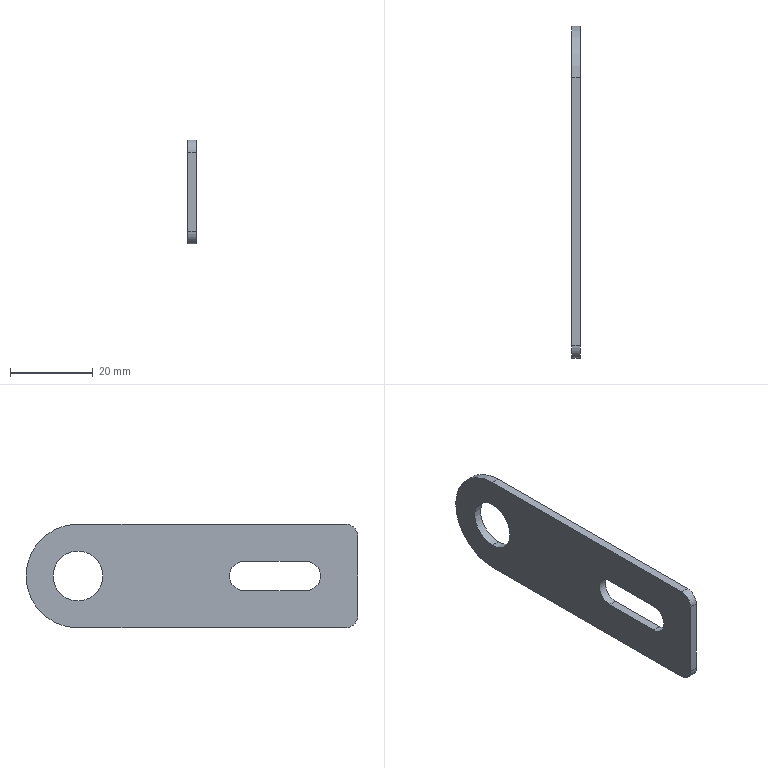Part | STEP file | Proximity switch bracket 1 | 1 solid | 15 faces | box 2 x 80 x 25 mm | volume 3345 mm3 | cylinder 8 | plane 7 | commonest cylinder face diameters 6 x2 7 x2 12 x2 25 x2
STEP:
#1=CARTESIAN_POINT('',(0.,0.,0.));
#2=DIRECTION('',(0.,0.,1.));
#3=DIRECTION('',(1.,0.,0.));
#4=AXIS2_PLACEMENT_3D('',#1,#2,#3);
#5=CARTESIAN_POINT('',(0.,67.5,6.));
#6=VERTEX_POINT('',#5);
#7=CARTESIAN_POINT('',(-2.,67.5,6.));
#8=VERTEX_POINT('',#7);
#9=CARTESIAN_POINT('',(-2.,67.5,6.));
#10=DIRECTION('',(-1.,0.,0.));
#11=VECTOR('',#10,1.);
#12=LINE('',#9,#11);
#13=CARTESIAN_POINT('',(-2.,67.5,0.));
#14=DIRECTION('',(-1.,0.,0.));
#15=DIRECTION('',(0.,0.,1.));
#16=AXIS2_PLACEMENT_3D('',#13,#14,#15);
#17=CYLINDRICAL_SURFACE('',#16,6.);
#18=CARTESIAN_POINT('',(6.283,0.));
#19=DIRECTION('',(0.,1.));
#20=VECTOR('',#19,1.);
#21=LINE('',#18,#20);
#22=(GEOMETRIC_REPRESENTATION_CONTEXT(2)PARAMETRIC_REPRESENTATION_CONTEXT()REPRESENTATION_CONTEXT('',''));
#23=DEFINITIONAL_REPRESENTATION('',(#21),#22);
#24=PCURVE('',#17,#23);
#25=CARTESIAN_POINT('',(-2.,67.5,0.));
#26=DIRECTION('',(-1.,0.,0.));
#27=DIRECTION('',(0.,0.,1.));
#28=AXIS2_PLACEMENT_3D('',#25,#26,#27);
#29=CYLINDRICAL_SURFACE('',#28,6.);
#30=CARTESIAN_POINT('',(0.,0.));
#31=DIRECTION('',(0.,1.));
#32=VECTOR('',#31,1.);
#33=LINE('',#30,#32);
#34=(GEOMETRIC_REPRESENTATION_CONTEXT(2)PARAMETRIC_REPRESENTATION_CONTEXT()REPRESENTATION_CONTEXT('',''));
#35=DEFINITIONAL_REPRESENTATION('',(#33),#34);
#36=PCURVE('',#29,#35);
#37=SURFACE_CURVE('',#12,(#24,#36),.PCURVE_S1.);
#38=EDGE_CURVE('',#6,#8,#37,.T.);
#39=ORIENTED_EDGE('',*,*,#38,.T.);
#40=CARTESIAN_POINT('',(-2.,67.5,-6.));
#41=VERTEX_POINT('',#40);
#42=CARTESIAN_POINT('',(-2.,67.5,0.));
#43=DIRECTION('',(-1.,0.,0.));
#44=DIRECTION('',(0.,0.,1.));
#45=AXIS2_PLACEMENT_3D('',#42,#43,#44);
#46=CIRCLE('',#45,6.);
#47=CARTESIAN_POINT('',(0.,0.));
#48=DIRECTION('',(1.,0.));
#49=VECTOR('',#48,1.);
#50=LINE('',#47,#49);
#51=(GEOMETRIC_REPRESENTATION_CONTEXT(2)PARAMETRIC_REPRESENTATION_CONTEXT()REPRESENTATION_CONTEXT('',''));
#52=DEFINITIONAL_REPRESENTATION('',(#50),#51);
#53=PCURVE('',#17,#52);
#54=CARTESIAN_POINT('',(-2.,0.,12.5));
#55=DIRECTION('',(1.,0.,0.));
#56=DIRECTION('',(0.,0.,-1.));
#57=AXIS2_PLACEMENT_3D('',#54,#55,#56);
#58=PLANE('',#57);
#59=CARTESIAN_POINT('',(6.5,67.5));
#60=CARTESIAN_POINT('',(6.5,77.892));
#61=CARTESIAN_POINT('',(15.5,72.696));
#62=CARTESIAN_POINT('',(24.5,67.5));
#63=CARTESIAN_POINT('',(15.5,62.304));
#64=CARTESIAN_POINT('',(6.5,57.108));
#65=CARTESIAN_POINT('',(6.5,67.5));
#66=(BOUNDED_CURVE()B_SPLINE_CURVE(2,(#59,#60,#61,#62,#63,#64,#65),.UNSPECIFIED.,.T.,.F.)B_SPLINE_CURVE_WITH_KNOTS((1,2,2,2,2,1),(-2.094,0.,2.094,4.189,6.283,8.378),.UNSPECIFIED.)CURVE()GEOMETRIC_REPRESENTATION_ITEM()RATIONAL_B_SPLINE_CURVE((1.,0.5,1.,0.5,1.,0.5,1.))REPRESENTATION_ITEM(''));
#67=(GEOMETRIC_REPRESENTATION_CONTEXT(2)PARAMETRIC_REPRESENTATION_CONTEXT()REPRESENTATION_CONTEXT('',''));
#68=DEFINITIONAL_REPRESENTATION('',(#66),#67);
#69=PCURVE('',#58,#68);
#70=SURFACE_CURVE('',#46,(#53,#69),.PCURVE_S1.);
#71=EDGE_CURVE('',#41,#8,#70,.T.);
#72=ORIENTED_EDGE('',*,*,#71,.F.);
#73=CARTESIAN_POINT('',(0.,67.5,-6.));
#74=VERTEX_POINT('',#73);
#75=CARTESIAN_POINT('',(-2.,67.5,-6.));
#76=DIRECTION('',(-1.,0.,0.));
#77=VECTOR('',#76,1.);
#78=LINE('',#75,#77);
#79=CARTESIAN_POINT('',(3.142,0.));
#80=DIRECTION('',(0.,1.));
#81=VECTOR('',#80,1.);
#82=LINE('',#79,#81);
#83=(GEOMETRIC_REPRESENTATION_CONTEXT(2)PARAMETRIC_REPRESENTATION_CONTEXT()REPRESENTATION_CONTEXT('',''));
#84=DEFINITIONAL_REPRESENTATION('',(#82),#83);
#85=PCURVE('',#17,#84);
#86=CARTESIAN_POINT('',(3.142,0.));
#87=DIRECTION('',(0.,1.));
#88=VECTOR('',#87,1.);
#89=LINE('',#86,#88);
#90=(GEOMETRIC_REPRESENTATION_CONTEXT(2)PARAMETRIC_REPRESENTATION_CONTEXT()REPRESENTATION_CONTEXT('',''));
#91=DEFINITIONAL_REPRESENTATION('',(#89),#90);
#92=PCURVE('',#29,#91);
#93=SURFACE_CURVE('',#78,(#85,#92),.PCURVE_S1.);
#94=EDGE_CURVE('',#74,#41,#93,.T.);
#95=ORIENTED_EDGE('',*,*,#94,.F.);
#96=CARTESIAN_POINT('',(0.,67.5,0.));
#97=DIRECTION('',(-1.,0.,0.));
#98=DIRECTION('',(0.,0.,1.));
#99=AXIS2_PLACEMENT_3D('',#96,#97,#98);
#100=CIRCLE('',#99,6.);
#101=CARTESIAN_POINT('',(0.,-2.));
#102=DIRECTION('',(1.,0.));
#103=VECTOR('',#102,1.);
#104=LINE('',#101,#103);
#105=(GEOMETRIC_REPRESENTATION_CONTEXT(2)PARAMETRIC_REPRESENTATION_CONTEXT()REPRESENTATION_CONTEXT('',''));
#106=DEFINITIONAL_REPRESENTATION('',(#104),#105);
#107=PCURVE('',#17,#106);
#108=CARTESIAN_POINT('',(0.,0.,12.5));
#109=DIRECTION('',(1.,0.,0.));
#110=DIRECTION('',(0.,0.,-1.));
#111=AXIS2_PLACEMENT_3D('',#108,#109,#110);
#112=PLANE('',#111);
#113=CARTESIAN_POINT('',(6.5,67.5));
#114=CARTESIAN_POINT('',(6.5,77.892));
#115=CARTESIAN_POINT('',(15.5,72.696));
#116=CARTESIAN_POINT('',(24.5,67.5));
#117=CARTESIAN_POINT('',(15.5,62.304));
#118=CARTESIAN_POINT('',(6.5,57.108));
#119=CARTESIAN_POINT('',(6.5,67.5));
#120=(BOUNDED_CURVE()B_SPLINE_CURVE(2,(#113,#114,#115,#116,#117,#118,#119),.UNSPECIFIED.,.T.,.F.)B_SPLINE_CURVE_WITH_KNOTS((1,2,2,2,2,1),(-2.094,0.,2.094,4.189,6.283,8.378),.UNSPECIFIED.)CURVE()GEOMETRIC_REPRESENTATION_ITEM()RATIONAL_B_SPLINE_CURVE((1.,0.5,1.,0.5,1.,0.5,1.))REPRESENTATION_ITEM(''));
#121=(GEOMETRIC_REPRESENTATION_CONTEXT(2)PARAMETRIC_REPRESENTATION_CONTEXT()REPRESENTATION_CONTEXT('',''));
#122=DEFINITIONAL_REPRESENTATION('',(#120),#121);
#123=PCURVE('',#112,#122);
#124=SURFACE_CURVE('',#100,(#107,#123),.PCURVE_S1.);
#125=EDGE_CURVE('',#74,#6,#124,.T.);
#126=ORIENTED_EDGE('',*,*,#125,.T.);
#127=EDGE_LOOP('',(#39,#72,#95,#126));
#128=FACE_BOUND('',#127,.F.);
#129=ADVANCED_FACE('',(#128),#17,.F.);
#130=CARTESIAN_POINT('',(-2.,12.5,3.5));
#131=VERTEX_POINT('',#130);
#132=CARTESIAN_POINT('',(-2.,27.5,3.5));
#133=VERTEX_POINT('',#132);
#134=CARTESIAN_POINT('',(-2.,12.5,3.5));
#135=DIRECTION('',(0.,1.,0.));
#136=VECTOR('',#135,1.);
#137=LINE('',#134,#136);
#138=CARTESIAN_POINT('',(9.,12.5));
#139=DIRECTION('',(0.,1.));
#140=VECTOR('',#139,1.);
#141=LINE('',#138,#140);
#142=(GEOMETRIC_REPRESENTATION_CONTEXT(2)PARAMETRIC_REPRESENTATION_CONTEXT()REPRESENTATION_CONTEXT('',''));
#143=DEFINITIONAL_REPRESENTATION('',(#141),#142);
#144=PCURVE('',#58,#143);
#145=CARTESIAN_POINT('',(0.,12.5,3.5));
#146=DIRECTION('',(0.,0.,1.));
#147=DIRECTION('',(0.,-1.,0.));
#148=AXIS2_PLACEMENT_3D('',#145,#146,#147);
#149=PLANE('',#148);
#150=CARTESIAN_POINT('',(0.,-2.));
#151=DIRECTION('',(-1.,0.));
#152=VECTOR('',#151,1.);
#153=LINE('',#150,#152);
#154=(GEOMETRIC_REPRESENTATION_CONTEXT(2)PARAMETRIC_REPRESENTATION_CONTEXT()REPRESENTATION_CONTEXT('',''));
#155=DEFINITIONAL_REPRESENTATION('',(#153),#154);
#156=PCURVE('',#149,#155);
#157=SURFACE_CURVE('',#137,(#144,#156),.PCURVE_S1.);
#158=EDGE_CURVE('',#131,#133,#157,.T.);
#159=ORIENTED_EDGE('',*,*,#158,.F.);
#160=CARTESIAN_POINT('',(-2.,12.5,-3.5));
#161=VERTEX_POINT('',#160);
#162=CARTESIAN_POINT('',(-2.,12.5,0.));
#163=DIRECTION('',(-1.,0.,0.));
#164=DIRECTION('',(0.,0.,1.));
#165=AXIS2_PLACEMENT_3D('',#162,#163,#164);
#166=CIRCLE('',#165,3.5);
#167=CARTESIAN_POINT('',(9.,12.5));
#168=CARTESIAN_POINT('',(9.,18.562));
#169=CARTESIAN_POINT('',(14.25,15.531));
#170=CARTESIAN_POINT('',(19.5,12.5));
#171=CARTESIAN_POINT('',(14.25,9.469));
#172=CARTESIAN_POINT('',(9.,6.438));
#173=CARTESIAN_POINT('',(9.,12.5));
#174=(BOUNDED_CURVE()B_SPLINE_CURVE(2,(#167,#168,#169,#170,#171,#172,#173),.UNSPECIFIED.,.T.,.F.)B_SPLINE_CURVE_WITH_KNOTS((1,2,2,2,2,1),(-2.094,0.,2.094,4.189,6.283,8.378),.UNSPECIFIED.)CURVE()GEOMETRIC_REPRESENTATION_ITEM()RATIONAL_B_SPLINE_CURVE((1.,0.5,1.,0.5,1.,0.5,1.))REPRESENTATION_ITEM(''));
#175=(GEOMETRIC_REPRESENTATION_CONTEXT(2)PARAMETRIC_REPRESENTATION_CONTEXT()REPRESENTATION_CONTEXT('',''));
#176=DEFINITIONAL_REPRESENTATION('',(#174),#175);
#177=PCURVE('',#58,#176);
#178=CARTESIAN_POINT('',(0.,12.5,0.));
#179=DIRECTION('',(-1.,0.,0.));
#180=DIRECTION('',(0.,0.,1.));
#181=AXIS2_PLACEMENT_3D('',#178,#179,#180);
#182=CYLINDRICAL_SURFACE('',#181,3.5);
#183=CARTESIAN_POINT('',(0.,2.));
#184=DIRECTION('',(1.,0.));
#185=VECTOR('',#184,1.);
#186=LINE('',#183,#185);
#187=(GEOMETRIC_REPRESENTATION_CONTEXT(2)PARAMETRIC_REPRESENTATION_CONTEXT()REPRESENTATION_CONTEXT('',''));
#188=DEFINITIONAL_REPRESENTATION('',(#186),#187);
#189=PCURVE('',#182,#188);
#190=SURFACE_CURVE('',#166,(#177,#189),.PCURVE_S1.);
#191=EDGE_CURVE('',#161,#131,#190,.T.);
#192=ORIENTED_EDGE('',*,*,#191,.F.);
#193=CARTESIAN_POINT('',(-2.,27.5,-3.5));
#194=VERTEX_POINT('',#193);
#195=CARTESIAN_POINT('',(-2.,12.5,-3.5));
#196=DIRECTION('',(0.,-1.,0.));
#197=VECTOR('',#196,1.);
#198=LINE('',#195,#197);
#199=CARTESIAN_POINT('',(16.,12.5));
#200=DIRECTION('',(0.,-1.));
#201=VECTOR('',#200,1.);
#202=LINE('',#199,#201);
#203=(GEOMETRIC_REPRESENTATION_CONTEXT(2)PARAMETRIC_REPRESENTATION_CONTEXT()REPRESENTATION_CONTEXT('',''));
#204=DEFINITIONAL_REPRESENTATION('',(#202),#203);
#205=PCURVE('',#58,#204);
#206=CARTESIAN_POINT('',(0.,12.5,-3.5));
#207=DIRECTION('',(0.,0.,-1.));
#208=DIRECTION('',(0.,1.,0.));
#209=AXIS2_PLACEMENT_3D('',#206,#207,#208);
#210=PLANE('',#209);
#211=CARTESIAN_POINT('',(0.,-2.));
#212=DIRECTION('',(-1.,0.));
#213=VECTOR('',#212,1.);
#214=LINE('',#211,#213);
#215=(GEOMETRIC_REPRESENTATION_CONTEXT(2)PARAMETRIC_REPRESENTATION_CONTEXT()REPRESENTATION_CONTEXT('',''));
#216=DEFINITIONAL_REPRESENTATION('',(#214),#215);
#217=PCURVE('',#210,#216);
#218=SURFACE_CURVE('',#198,(#205,#217),.PCURVE_S1.);
#219=EDGE_CURVE('',#194,#161,#218,.T.);
#220=ORIENTED_EDGE('',*,*,#219,.F.);
#221=CARTESIAN_POINT('',(-2.,27.5,0.));
#222=DIRECTION('',(-1.,0.,0.));
#223=DIRECTION('',(0.,0.,1.));
#224=AXIS2_PLACEMENT_3D('',#221,#222,#223);
#225=CIRCLE('',#224,3.5);
#226=CARTESIAN_POINT('',(9.,27.5));
#227=CARTESIAN_POINT('',(9.,33.562));
#228=CARTESIAN_POINT('',(14.25,30.531));
#229=CARTESIAN_POINT('',(19.5,27.5));
#230=CARTESIAN_POINT('',(14.25,24.469));
#231=CARTESIAN_POINT('',(9.,21.438));
#232=CARTESIAN_POINT('',(9.,27.5));
#233=(BOUNDED_CURVE()B_SPLINE_CURVE(2,(#226,#227,#228,#229,#230,#231,#232),.UNSPECIFIED.,.T.,.F.)B_SPLINE_CURVE_WITH_KNOTS((1,2,2,2,2,1),(-2.094,0.,2.094,4.189,6.283,8.378),.UNSPECIFIED.)CURVE()GEOMETRIC_REPRESENTATION_ITEM()RATIONAL_B_SPLINE_CURVE((1.,0.5,1.,0.5,1.,0.5,1.))REPRESENTATION_ITEM(''));
#234=(GEOMETRIC_REPRESENTATION_CONTEXT(2)PARAMETRIC_REPRESENTATION_CONTEXT()REPRESENTATION_CONTEXT('',''));
#235=DEFINITIONAL_REPRESENTATION('',(#233),#234);
#236=PCURVE('',#58,#235);
#237=CARTESIAN_POINT('',(0.,27.5,0.));
#238=DIRECTION('',(-1.,0.,0.));
#239=DIRECTION('',(0.,0.,1.));
#240=AXIS2_PLACEMENT_3D('',#237,#238,#239);
#241=CYLINDRICAL_SURFACE('',#240,3.5);
#242=CARTESIAN_POINT('',(0.,2.));
#243=DIRECTION('',(1.,0.));
#244=VECTOR('',#243,1.);
#245=LINE('',#242,#244);
#246=(GEOMETRIC_REPRESENTATION_CONTEXT(2)PARAMETRIC_REPRESENTATION_CONTEXT()REPRESENTATION_CONTEXT('',''));
#247=DEFINITIONAL_REPRESENTATION('',(#245),#246);
#248=PCURVE('',#241,#247);
#249=SURFACE_CURVE('',#225,(#236,#248),.PCURVE_S1.);
#250=EDGE_CURVE('',#133,#194,#249,.T.);
#251=ORIENTED_EDGE('',*,*,#250,.F.);
#252=EDGE_LOOP('',(#159,#192,#220,#251));
#253=FACE_BOUND('',#252,.T.);
#254=CARTESIAN_POINT('',(-2.,67.5,0.));
#255=DIRECTION('',(-1.,0.,0.));
#256=DIRECTION('',(0.,0.,1.));
#257=AXIS2_PLACEMENT_3D('',#254,#255,#256);
#258=CIRCLE('',#257,6.);
#259=CARTESIAN_POINT('',(6.5,67.5));
#260=CARTESIAN_POINT('',(6.5,77.892));
#261=CARTESIAN_POINT('',(15.5,72.696));
#262=CARTESIAN_POINT('',(24.5,67.5));
#263=CARTESIAN_POINT('',(15.5,62.304));
#264=CARTESIAN_POINT('',(6.5,57.108));
#265=CARTESIAN_POINT('',(6.5,67.5));
#266=(BOUNDED_CURVE()B_SPLINE_CURVE(2,(#259,#260,#261,#262,#263,#264,#265),.UNSPECIFIED.,.T.,.F.)B_SPLINE_CURVE_WITH_KNOTS((1,2,2,2,2,1),(-2.094,0.,2.094,4.189,6.283,8.378),.UNSPECIFIED.)CURVE()GEOMETRIC_REPRESENTATION_ITEM()RATIONAL_B_SPLINE_CURVE((1.,0.5,1.,0.5,1.,0.5,1.))REPRESENTATION_ITEM(''));
#267=(GEOMETRIC_REPRESENTATION_CONTEXT(2)PARAMETRIC_REPRESENTATION_CONTEXT()REPRESENTATION_CONTEXT('',''));
#268=DEFINITIONAL_REPRESENTATION('',(#266),#267);
#269=PCURVE('',#58,#268);
#270=CARTESIAN_POINT('',(0.,0.));
#271=DIRECTION('',(1.,0.));
#272=VECTOR('',#271,1.);
#273=LINE('',#270,#272);
#274=(GEOMETRIC_REPRESENTATION_CONTEXT(2)PARAMETRIC_REPRESENTATION_CONTEXT()REPRESENTATION_CONTEXT('',''));
#275=DEFINITIONAL_REPRESENTATION('',(#273),#274);
#276=PCURVE('',#29,#275);
#277=SURFACE_CURVE('',#258,(#269,#276),.PCURVE_S1.);
#278=EDGE_CURVE('',#8,#41,#277,.T.);
#279=ORIENTED_EDGE('',*,*,#278,.F.);
#280=ORIENTED_EDGE('',*,*,#71,.F.);
#281=EDGE_LOOP('',(#279,#280));
#282=FACE_BOUND('',#281,.T.);
#283=CARTESIAN_POINT('',(-2.,0.,9.5));
#284=VERTEX_POINT('',#283);
#285=CARTESIAN_POINT('',(-2.,0.,-9.5));
#286=VERTEX_POINT('',#285);
#287=CARTESIAN_POINT('',(-2.,0.,12.5));
#288=DIRECTION('',(0.,0.,-1.));
#289=VECTOR('',#288,1.);
#290=LINE('',#287,#289);
#291=CARTESIAN_POINT('',(0.,0.));
#292=DIRECTION('',(1.,0.));
#293=VECTOR('',#292,1.);
#294=LINE('',#291,#293);
#295=(GEOMETRIC_REPRESENTATION_CONTEXT(2)PARAMETRIC_REPRESENTATION_CONTEXT()REPRESENTATION_CONTEXT('',''));
#296=DEFINITIONAL_REPRESENTATION('',(#294),#295);
#297=PCURVE('',#58,#296);
#298=CARTESIAN_POINT('',(0.,0.,12.5));
#299=DIRECTION('',(0.,-1.,0.));
#300=DIRECTION('',(0.,0.,-1.));
#301=AXIS2_PLACEMENT_3D('',#298,#299,#300);
#302=PLANE('',#301);
#303=CARTESIAN_POINT('',(0.,-2.));
#304=DIRECTION('',(1.,0.));
#305=VECTOR('',#304,1.);
#306=LINE('',#303,#305);
#307=(GEOMETRIC_REPRESENTATION_CONTEXT(2)PARAMETRIC_REPRESENTATION_CONTEXT()REPRESENTATION_CONTEXT('',''));
#308=DEFINITIONAL_REPRESENTATION('',(#306),#307);
#309=PCURVE('',#302,#308);
#310=SURFACE_CURVE('',#290,(#297,#309),.PCURVE_S1.);
#311=EDGE_CURVE('',#284,#286,#310,.T.);
#312=ORIENTED_EDGE('',*,*,#311,.F.);
#313=CARTESIAN_POINT('',(-2.,3.,12.5));
#314=VERTEX_POINT('',#313);
#315=CARTESIAN_POINT('',(-2.,3.,9.5));
#316=DIRECTION('',(-1.,0.,0.));
#317=DIRECTION('',(0.,0.,-1.));
#318=AXIS2_PLACEMENT_3D('',#315,#316,#317);
#319=CIRCLE('',#318,3.);
#320=CARTESIAN_POINT('',(6.,3.));
#321=CARTESIAN_POINT('',(6.,-2.196));
#322=CARTESIAN_POINT('',(1.5,0.4019));
#323=CARTESIAN_POINT('',(-3.,3.));
#324=CARTESIAN_POINT('',(1.5,5.598));
#325=CARTESIAN_POINT('',(6.,8.196));
#326=CARTESIAN_POINT('',(6.,3.));
#327=(BOUNDED_CURVE()B_SPLINE_CURVE(2,(#320,#321,#322,#323,#324,#325,#326),.UNSPECIFIED.,.T.,.F.)B_SPLINE_CURVE_WITH_KNOTS((1,2,2,2,2,1),(-2.094,0.,2.094,4.189,6.283,8.378),.UNSPECIFIED.)CURVE()GEOMETRIC_REPRESENTATION_ITEM()RATIONAL_B_SPLINE_CURVE((1.,0.5,1.,0.5,1.,0.5,1.))REPRESENTATION_ITEM(''));
#328=(GEOMETRIC_REPRESENTATION_CONTEXT(2)PARAMETRIC_REPRESENTATION_CONTEXT()REPRESENTATION_CONTEXT('',''));
#329=DEFINITIONAL_REPRESENTATION('',(#327),#328);
#330=PCURVE('',#58,#329);
#331=CARTESIAN_POINT('',(0.,3.,9.5));
#332=DIRECTION('',(-1.,0.,0.));
#333=DIRECTION('',(0.,0.,1.));
#334=AXIS2_PLACEMENT_3D('',#331,#332,#333);
#335=CYLINDRICAL_SURFACE('',#334,3.);
#336=CARTESIAN_POINT('',(3.142,2.));
#337=DIRECTION('',(1.,0.));
#338=VECTOR('',#337,1.);
#339=LINE('',#336,#338);
#340=(GEOMETRIC_REPRESENTATION_CONTEXT(2)PARAMETRIC_REPRESENTATION_CONTEXT()REPRESENTATION_CONTEXT('',''));
#341=DEFINITIONAL_REPRESENTATION('',(#339),#340);
#342=PCURVE('',#335,#341);
#343=SURFACE_CURVE('',#319,(#330,#342),.PCURVE_S1.);
#344=EDGE_CURVE('',#284,#314,#343,.T.);
#345=ORIENTED_EDGE('',*,*,#344,.T.);
#346=CARTESIAN_POINT('',(-2.,67.5,12.5));
#347=VERTEX_POINT('',#346);
#348=CARTESIAN_POINT('',(-2.,0.,12.5));
#349=DIRECTION('',(0.,-1.,0.));
#350=VECTOR('',#349,1.);
#351=LINE('',#348,#350);
#352=CARTESIAN_POINT('',(0.,0.));
#353=DIRECTION('',(0.,-1.));
#354=VECTOR('',#353,1.);
#355=LINE('',#352,#354);
#356=(GEOMETRIC_REPRESENTATION_CONTEXT(2)PARAMETRIC_REPRESENTATION_CONTEXT()REPRESENTATION_CONTEXT('',''));
#357=DEFINITIONAL_REPRESENTATION('',(#355),#356);
#358=PCURVE('',#58,#357);
#359=CARTESIAN_POINT('',(0.,0.,12.5));
#360=DIRECTION('',(0.,0.,1.));
#361=DIRECTION('',(1.,0.,0.));
#362=AXIS2_PLACEMENT_3D('',#359,#360,#361);
#363=PLANE('',#362);
#364=CARTESIAN_POINT('',(-2.,0.));
#365=DIRECTION('',(0.,-1.));
#366=VECTOR('',#365,1.);
#367=LINE('',#364,#366);
#368=(GEOMETRIC_REPRESENTATION_CONTEXT(2)PARAMETRIC_REPRESENTATION_CONTEXT()REPRESENTATION_CONTEXT('',''));
#369=DEFINITIONAL_REPRESENTATION('',(#367),#368);
#370=PCURVE('',#363,#369);
#371=SURFACE_CURVE('',#351,(#358,#370),.PCURVE_S1.);
#372=EDGE_CURVE('',#347,#314,#371,.T.);
#373=ORIENTED_EDGE('',*,*,#372,.F.);
#374=CARTESIAN_POINT('',(-2.,80.,0.));
#375=VERTEX_POINT('',#374);
#376=CARTESIAN_POINT('',(-2.,67.5,0.));
#377=DIRECTION('',(-1.,0.,0.));
#378=DIRECTION('',(0.,0.,-1.));
#379=AXIS2_PLACEMENT_3D('',#376,#377,#378);
#380=CIRCLE('',#379,12.5);
#381=CARTESIAN_POINT('',(25.,67.5));
#382=CARTESIAN_POINT('',(25.,45.849));
#383=CARTESIAN_POINT('',(6.25,56.675));
#384=CARTESIAN_POINT('',(-12.5,67.5));
#385=CARTESIAN_POINT('',(6.25,78.325));
#386=CARTESIAN_POINT('',(25.,89.151));
#387=CARTESIAN_POINT('',(25.,67.5));
#388=(BOUNDED_CURVE()B_SPLINE_CURVE(2,(#381,#382,#383,#384,#385,#386,#387),.UNSPECIFIED.,.T.,.F.)B_SPLINE_CURVE_WITH_KNOTS((1,2,2,2,2,1),(-2.094,0.,2.094,4.189,6.283,8.378),.UNSPECIFIED.)CURVE()GEOMETRIC_REPRESENTATION_ITEM()RATIONAL_B_SPLINE_CURVE((1.,0.5,1.,0.5,1.,0.5,1.))REPRESENTATION_ITEM(''));
#389=(GEOMETRIC_REPRESENTATION_CONTEXT(2)PARAMETRIC_REPRESENTATION_CONTEXT()REPRESENTATION_CONTEXT('',''));
#390=DEFINITIONAL_REPRESENTATION('',(#388),#389);
#391=PCURVE('',#58,#390);
#392=CARTESIAN_POINT('',(-2.,67.5,0.));
#393=DIRECTION('',(1.,0.,0.));
#394=DIRECTION('',(0.,0.,-1.));
#395=AXIS2_PLACEMENT_3D('',#392,#393,#394);
#396=CYLINDRICAL_SURFACE('',#395,12.5);
#397=CARTESIAN_POINT('',(6.283,0.));
#398=DIRECTION('',(-1.,0.));
#399=VECTOR('',#398,1.);
#400=LINE('',#397,#399);
#401=(GEOMETRIC_REPRESENTATION_CONTEXT(2)PARAMETRIC_REPRESENTATION_CONTEXT()REPRESENTATION_CONTEXT('',''));
#402=DEFINITIONAL_REPRESENTATION('',(#400),#401);
#403=PCURVE('',#396,#402);
#404=SURFACE_CURVE('',#380,(#391,#403),.PCURVE_S1.);
#405=EDGE_CURVE('',#347,#375,#404,.T.);
#406=ORIENTED_EDGE('',*,*,#405,.T.);
#407=CARTESIAN_POINT('',(-2.,67.5,-12.5));
#408=VERTEX_POINT('',#407);
#409=CARTESIAN_POINT('',(-2.,67.5,0.));
#410=DIRECTION('',(-1.,0.,0.));
#411=DIRECTION('',(0.,0.,-1.));
#412=AXIS2_PLACEMENT_3D('',#409,#410,#411);
#413=CIRCLE('',#412,12.5);
#414=CARTESIAN_POINT('',(25.,67.5));
#415=CARTESIAN_POINT('',(25.,45.849));
#416=CARTESIAN_POINT('',(6.25,56.675));
#417=CARTESIAN_POINT('',(-12.5,67.5));
#418=CARTESIAN_POINT('',(6.25,78.325));
#419=CARTESIAN_POINT('',(25.,89.151));
#420=CARTESIAN_POINT('',(25.,67.5));
#421=(BOUNDED_CURVE()B_SPLINE_CURVE(2,(#414,#415,#416,#417,#418,#419,#420),.UNSPECIFIED.,.T.,.F.)B_SPLINE_CURVE_WITH_KNOTS((1,2,2,2,2,1),(-2.094,0.,2.094,4.189,6.283,8.378),.UNSPECIFIED.)CURVE()GEOMETRIC_REPRESENTATION_ITEM()RATIONAL_B_SPLINE_CURVE((1.,0.5,1.,0.5,1.,0.5,1.))REPRESENTATION_ITEM(''));
#422=(GEOMETRIC_REPRESENTATION_CONTEXT(2)PARAMETRIC_REPRESENTATION_CONTEXT()REPRESENTATION_CONTEXT('',''));
#423=DEFINITIONAL_REPRESENTATION('',(#421),#422);
#424=PCURVE('',#58,#423);
#425=CARTESIAN_POINT('',(0.,67.5,0.));
#426=DIRECTION('',(-1.,0.,0.));
#427=DIRECTION('',(0.,0.,1.));
#428=AXIS2_PLACEMENT_3D('',#425,#426,#427);
#429=CYLINDRICAL_SURFACE('',#428,12.5);
#430=CARTESIAN_POINT('',(-3.142,2.));
#431=DIRECTION('',(1.,0.));
#432=VECTOR('',#431,1.);
#433=LINE('',#430,#432);
#434=(GEOMETRIC_REPRESENTATION_CONTEXT(2)PARAMETRIC_REPRESENTATION_CONTEXT()REPRESENTATION_CONTEXT('',''));
#435=DEFINITIONAL_REPRESENTATION('',(#433),#434);
#436=PCURVE('',#429,#435);
#437=SURFACE_CURVE('',#413,(#424,#436),.PCURVE_S1.);
#438=EDGE_CURVE('',#375,#408,#437,.T.);
#439=ORIENTED_EDGE('',*,*,#438,.T.);
#440=CARTESIAN_POINT('',(-2.,3.,-12.5));
#441=VERTEX_POINT('',#440);
#442=CARTESIAN_POINT('',(-2.,0.,-12.5));
#443=DIRECTION('',(0.,-1.,0.));
#444=VECTOR('',#443,1.);
#445=LINE('',#442,#444);
#446=CARTESIAN_POINT('',(25.,0.));
#447=DIRECTION('',(0.,-1.));
#448=VECTOR('',#447,1.);
#449=LINE('',#446,#448);
#450=(GEOMETRIC_REPRESENTATION_CONTEXT(2)PARAMETRIC_REPRESENTATION_CONTEXT()REPRESENTATION_CONTEXT('',''));
#451=DEFINITIONAL_REPRESENTATION('',(#449),#450);
#452=PCURVE('',#58,#451);
#453=CARTESIAN_POINT('',(0.,0.,-12.5));
#454=DIRECTION('',(0.,0.,1.));
#455=DIRECTION('',(1.,0.,0.));
#456=AXIS2_PLACEMENT_3D('',#453,#454,#455);
#457=PLANE('',#456);
#458=CARTESIAN_POINT('',(-2.,0.));
#459=DIRECTION('',(0.,-1.));
#460=VECTOR('',#459,1.);
#461=LINE('',#458,#460);
#462=(GEOMETRIC_REPRESENTATION_CONTEXT(2)PARAMETRIC_REPRESENTATION_CONTEXT()REPRESENTATION_CONTEXT('',''));
#463=DEFINITIONAL_REPRESENTATION('',(#461),#462);
#464=PCURVE('',#457,#463);
#465=SURFACE_CURVE('',#445,(#452,#464),.PCURVE_S1.);
#466=EDGE_CURVE('',#408,#441,#465,.T.);
#467=ORIENTED_EDGE('',*,*,#466,.T.);
#468=CARTESIAN_POINT('',(-2.,3.,-9.5));
#469=DIRECTION('',(-1.,0.,0.));
#470=DIRECTION('',(0.,0.,-1.));
#471=AXIS2_PLACEMENT_3D('',#468,#469,#470);
#472=CIRCLE('',#471,3.);
#473=CARTESIAN_POINT('',(25.,3.));
#474=CARTESIAN_POINT('',(25.,-2.196));
#475=CARTESIAN_POINT('',(20.5,0.4019));
#476=CARTESIAN_POINT('',(16.,3.));
#477=CARTESIAN_POINT('',(20.5,5.598));
#478=CARTESIAN_POINT('',(25.,8.196));
#479=CARTESIAN_POINT('',(25.,3.));
#480=(BOUNDED_CURVE()B_SPLINE_CURVE(2,(#473,#474,#475,#476,#477,#478,#479),.UNSPECIFIED.,.T.,.F.)B_SPLINE_CURVE_WITH_KNOTS((1,2,2,2,2,1),(-2.094,0.,2.094,4.189,6.283,8.378),.UNSPECIFIED.)CURVE()GEOMETRIC_REPRESENTATION_ITEM()RATIONAL_B_SPLINE_CURVE((1.,0.5,1.,0.5,1.,0.5,1.))REPRESENTATION_ITEM(''));
#481=(GEOMETRIC_REPRESENTATION_CONTEXT(2)PARAMETRIC_REPRESENTATION_CONTEXT()REPRESENTATION_CONTEXT('',''));
#482=DEFINITIONAL_REPRESENTATION('',(#480),#481);
#483=PCURVE('',#58,#482);
#484=CARTESIAN_POINT('',(0.,3.,-9.5));
#485=DIRECTION('',(1.,0.,0.));
#486=DIRECTION('',(0.,0.,-1.));
#487=AXIS2_PLACEMENT_3D('',#484,#485,#486);
#488=CYLINDRICAL_SURFACE('',#487,3.);
#489=CARTESIAN_POINT('',(6.283,-2.));
#490=DIRECTION('',(-1.,0.));
#491=VECTOR('',#490,1.);
#492=LINE('',#489,#491);
#493=(GEOMETRIC_REPRESENTATION_CONTEXT(2)PARAMETRIC_REPRESENTATION_CONTEXT()REPRESENTATION_CONTEXT('',''));
#494=DEFINITIONAL_REPRESENTATION('',(#492),#493);
#495=PCURVE('',#488,#494);
#496=SURFACE_CURVE('',#472,(#483,#495),.PCURVE_S1.);
#497=EDGE_CURVE('',#441,#286,#496,.T.);
#498=ORIENTED_EDGE('',*,*,#497,.T.);
#499=EDGE_LOOP('',(#312,#345,#373,#406,#439,#467,#498));
#500=FACE_BOUND('',#499,.T.);
#501=ADVANCED_FACE('',(#253,#282,#500),#58,.F.);
#502=CARTESIAN_POINT('',(0.,0.,9.5));
#503=VERTEX_POINT('',#502);
#504=CARTESIAN_POINT('',(0.,0.,-9.5));
#505=VERTEX_POINT('',#504);
#506=CARTESIAN_POINT('',(0.,0.,12.5));
#507=DIRECTION('',(0.,0.,-1.));
#508=VECTOR('',#507,1.);
#509=LINE('',#506,#508);
#510=CARTESIAN_POINT('',(0.,0.));
#511=DIRECTION('',(1.,0.));
#512=VECTOR('',#511,1.);
#513=LINE('',#510,#512);
#514=(GEOMETRIC_REPRESENTATION_CONTEXT(2)PARAMETRIC_REPRESENTATION_CONTEXT()REPRESENTATION_CONTEXT('',''));
#515=DEFINITIONAL_REPRESENTATION('',(#513),#514);
#516=PCURVE('',#302,#515);
#517=CARTESIAN_POINT('',(0.,0.));
#518=DIRECTION('',(1.,0.));
#519=VECTOR('',#518,1.);
#520=LINE('',#517,#519);
#521=(GEOMETRIC_REPRESENTATION_CONTEXT(2)PARAMETRIC_REPRESENTATION_CONTEXT()REPRESENTATION_CONTEXT('',''));
#522=DEFINITIONAL_REPRESENTATION('',(#520),#521);
#523=PCURVE('',#112,#522);
#524=SURFACE_CURVE('',#509,(#516,#523),.PCURVE_S1.);
#525=EDGE_CURVE('',#503,#505,#524,.T.);
#526=ORIENTED_EDGE('',*,*,#525,.F.);
#527=CARTESIAN_POINT('',(0.,0.,9.5));
#528=DIRECTION('',(-1.,0.,0.));
#529=VECTOR('',#528,1.);
#530=LINE('',#527,#529);
#531=CARTESIAN_POINT('',(3.,0.));
#532=DIRECTION('',(0.,-1.));
#533=VECTOR('',#532,1.);
#534=LINE('',#531,#533);
#535=(GEOMETRIC_REPRESENTATION_CONTEXT(2)PARAMETRIC_REPRESENTATION_CONTEXT()REPRESENTATION_CONTEXT('',''));
#536=DEFINITIONAL_REPRESENTATION('',(#534),#535);
#537=PCURVE('',#302,#536);
#538=CARTESIAN_POINT('',(4.712,0.));
#539=DIRECTION('',(0.,1.));
#540=VECTOR('',#539,1.);
#541=LINE('',#538,#540);
#542=(GEOMETRIC_REPRESENTATION_CONTEXT(2)PARAMETRIC_REPRESENTATION_CONTEXT()REPRESENTATION_CONTEXT('',''));
#543=DEFINITIONAL_REPRESENTATION('',(#541),#542);
#544=PCURVE('',#335,#543);
#545=SURFACE_CURVE('',#530,(#537,#544),.PCURVE_S1.);
#546=EDGE_CURVE('',#503,#284,#545,.T.);
#547=ORIENTED_EDGE('',*,*,#546,.T.);
#548=ORIENTED_EDGE('',*,*,#311,.T.);
#549=CARTESIAN_POINT('',(0.,0.,-9.5));
#550=DIRECTION('',(1.,0.,0.));
#551=VECTOR('',#550,1.);
#552=LINE('',#549,#551);
#553=CARTESIAN_POINT('',(22.,0.));
#554=DIRECTION('',(0.,1.));
#555=VECTOR('',#554,1.);
#556=LINE('',#553,#555);
#557=(GEOMETRIC_REPRESENTATION_CONTEXT(2)PARAMETRIC_REPRESENTATION_CONTEXT()REPRESENTATION_CONTEXT('',''));
#558=DEFINITIONAL_REPRESENTATION('',(#556),#557);
#559=PCURVE('',#302,#558);
#560=CARTESIAN_POINT('',(4.712,0.));
#561=DIRECTION('',(0.,1.));
#562=VECTOR('',#561,1.);
#563=LINE('',#560,#562);
#564=(GEOMETRIC_REPRESENTATION_CONTEXT(2)PARAMETRIC_REPRESENTATION_CONTEXT()REPRESENTATION_CONTEXT('',''));
#565=DEFINITIONAL_REPRESENTATION('',(#563),#564);
#566=PCURVE('',#488,#565);
#567=SURFACE_CURVE('',#552,(#559,#566),.PCURVE_S1.);
#568=EDGE_CURVE('',#286,#505,#567,.T.);
#569=ORIENTED_EDGE('',*,*,#568,.T.);
#570=EDGE_LOOP('',(#526,#547,#548,#569));
#571=FACE_BOUND('',#570,.T.);
#572=ADVANCED_FACE('',(#571),#302,.T.);
#573=CARTESIAN_POINT('',(0.,12.5,-3.5));
#574=VERTEX_POINT('',#573);
#575=CARTESIAN_POINT('',(0.,12.5,3.5));
#576=VERTEX_POINT('',#575);
#577=CARTESIAN_POINT('',(0.,12.5,0.));
#578=DIRECTION('',(-1.,0.,0.));
#579=DIRECTION('',(0.,0.,1.));
#580=AXIS2_PLACEMENT_3D('',#577,#578,#579);
#581=CIRCLE('',#580,3.5);
#582=CARTESIAN_POINT('',(9.,12.5));
#583=CARTESIAN_POINT('',(9.,18.562));
#584=CARTESIAN_POINT('',(14.25,15.531));
#585=CARTESIAN_POINT('',(19.5,12.5));
#586=CARTESIAN_POINT('',(14.25,9.469));
#587=CARTESIAN_POINT('',(9.,6.438));
#588=CARTESIAN_POINT('',(9.,12.5));
#589=(BOUNDED_CURVE()B_SPLINE_CURVE(2,(#582,#583,#584,#585,#586,#587,#588),.UNSPECIFIED.,.T.,.F.)B_SPLINE_CURVE_WITH_KNOTS((1,2,2,2,2,1),(-2.094,0.,2.094,4.189,6.283,8.378),.UNSPECIFIED.)CURVE()GEOMETRIC_REPRESENTATION_ITEM()RATIONAL_B_SPLINE_CURVE((1.,0.5,1.,0.5,1.,0.5,1.))REPRESENTATION_ITEM(''));
#590=(GEOMETRIC_REPRESENTATION_CONTEXT(2)PARAMETRIC_REPRESENTATION_CONTEXT()REPRESENTATION_CONTEXT('',''));
#591=DEFINITIONAL_REPRESENTATION('',(#589),#590);
#592=PCURVE('',#112,#591);
#593=CARTESIAN_POINT('',(0.,0.));
#594=DIRECTION('',(1.,0.));
#595=VECTOR('',#594,1.);
#596=LINE('',#593,#595);
#597=(GEOMETRIC_REPRESENTATION_CONTEXT(2)PARAMETRIC_REPRESENTATION_CONTEXT()REPRESENTATION_CONTEXT('',''));
#598=DEFINITIONAL_REPRESENTATION('',(#596),#597);
#599=PCURVE('',#182,#598);
#600=SURFACE_CURVE('',#581,(#592,#599),.PCURVE_S1.);
#601=EDGE_CURVE('',#574,#576,#600,.T.);
#602=ORIENTED_EDGE('',*,*,#601,.T.);
#603=CARTESIAN_POINT('',(0.,27.5,3.5));
#604=VERTEX_POINT('',#603);
#605=CARTESIAN_POINT('',(0.,12.5,3.5));
#606=DIRECTION('',(0.,1.,0.));
#607=VECTOR('',#606,1.);
#608=LINE('',#605,#607);
#609=CARTESIAN_POINT('',(9.,12.5));
#610=DIRECTION('',(0.,1.));
#611=VECTOR('',#610,1.);
#612=LINE('',#609,#611);
#613=(GEOMETRIC_REPRESENTATION_CONTEXT(2)PARAMETRIC_REPRESENTATION_CONTEXT()REPRESENTATION_CONTEXT('',''));
#614=DEFINITIONAL_REPRESENTATION('',(#612),#613);
#615=PCURVE('',#112,#614);
#616=CARTESIAN_POINT('',(0.,0.));
#617=DIRECTION('',(-1.,0.));
#618=VECTOR('',#617,1.);
#619=LINE('',#616,#618);
#620=(GEOMETRIC_REPRESENTATION_CONTEXT(2)PARAMETRIC_REPRESENTATION_CONTEXT()REPRESENTATION_CONTEXT('',''));
#621=DEFINITIONAL_REPRESENTATION('',(#619),#620);
#622=PCURVE('',#149,#621);
#623=SURFACE_CURVE('',#608,(#615,#622),.PCURVE_S1.);
#624=EDGE_CURVE('',#576,#604,#623,.T.);
#625=ORIENTED_EDGE('',*,*,#624,.T.);
#626=CARTESIAN_POINT('',(0.,27.5,-3.5));
#627=VERTEX_POINT('',#626);
#628=CARTESIAN_POINT('',(0.,27.5,0.));
#629=DIRECTION('',(-1.,0.,0.));
#630=DIRECTION('',(0.,0.,1.));
#631=AXIS2_PLACEMENT_3D('',#628,#629,#630);
#632=CIRCLE('',#631,3.5);
#633=CARTESIAN_POINT('',(9.,27.5));
#634=CARTESIAN_POINT('',(9.,33.562));
#635=CARTESIAN_POINT('',(14.25,30.531));
#636=CARTESIAN_POINT('',(19.5,27.5));
#637=CARTESIAN_POINT('',(14.25,24.469));
#638=CARTESIAN_POINT('',(9.,21.438));
#639=CARTESIAN_POINT('',(9.,27.5));
#640=(BOUNDED_CURVE()B_SPLINE_CURVE(2,(#633,#634,#635,#636,#637,#638,#639),.UNSPECIFIED.,.T.,.F.)B_SPLINE_CURVE_WITH_KNOTS((1,2,2,2,2,1),(-2.094,0.,2.094,4.189,6.283,8.378),.UNSPECIFIED.)CURVE()GEOMETRIC_REPRESENTATION_ITEM()RATIONAL_B_SPLINE_CURVE((1.,0.5,1.,0.5,1.,0.5,1.))REPRESENTATION_ITEM(''));
#641=(GEOMETRIC_REPRESENTATION_CONTEXT(2)PARAMETRIC_REPRESENTATION_CONTEXT()REPRESENTATION_CONTEXT('',''));
#642=DEFINITIONAL_REPRESENTATION('',(#640),#641);
#643=PCURVE('',#112,#642);
#644=CARTESIAN_POINT('',(0.,0.));
#645=DIRECTION('',(1.,0.));
#646=VECTOR('',#645,1.);
#647=LINE('',#644,#646);
#648=(GEOMETRIC_REPRESENTATION_CONTEXT(2)PARAMETRIC_REPRESENTATION_CONTEXT()REPRESENTATION_CONTEXT('',''));
#649=DEFINITIONAL_REPRESENTATION('',(#647),#648);
#650=PCURVE('',#241,#649);
#651=SURFACE_CURVE('',#632,(#643,#650),.PCURVE_S1.);
#652=EDGE_CURVE('',#604,#627,#651,.T.);
#653=ORIENTED_EDGE('',*,*,#652,.T.);
#654=CARTESIAN_POINT('',(0.,12.5,-3.5));
#655=DIRECTION('',(0.,-1.,0.));
#656=VECTOR('',#655,1.);
#657=LINE('',#654,#656);
#658=CARTESIAN_POINT('',(16.,12.5));
#659=DIRECTION('',(0.,-1.));
#660=VECTOR('',#659,1.);
#661=LINE('',#658,#660);
#662=(GEOMETRIC_REPRESENTATION_CONTEXT(2)PARAMETRIC_REPRESENTATION_CONTEXT()REPRESENTATION_CONTEXT('',''));
#663=DEFINITIONAL_REPRESENTATION('',(#661),#662);
#664=PCURVE('',#112,#663);
#665=CARTESIAN_POINT('',(0.,0.));
#666=DIRECTION('',(-1.,0.));
#667=VECTOR('',#666,1.);
#668=LINE('',#665,#667);
#669=(GEOMETRIC_REPRESENTATION_CONTEXT(2)PARAMETRIC_REPRESENTATION_CONTEXT()REPRESENTATION_CONTEXT('',''));
#670=DEFINITIONAL_REPRESENTATION('',(#668),#669);
#671=PCURVE('',#210,#670);
#672=SURFACE_CURVE('',#657,(#664,#671),.PCURVE_S1.);
#673=EDGE_CURVE('',#627,#574,#672,.T.);
#674=ORIENTED_EDGE('',*,*,#673,.T.);
#675=EDGE_LOOP('',(#602,#625,#653,#674));
#676=FACE_BOUND('',#675,.T.);
#677=CARTESIAN_POINT('',(0.,67.5,0.));
#678=DIRECTION('',(-1.,0.,0.));
#679=DIRECTION('',(0.,0.,1.));
#680=AXIS2_PLACEMENT_3D('',#677,#678,#679);
#681=CIRCLE('',#680,6.);
#682=CARTESIAN_POINT('',(6.5,67.5));
#683=CARTESIAN_POINT('',(6.5,77.892));
#684=CARTESIAN_POINT('',(15.5,72.696));
#685=CARTESIAN_POINT('',(24.5,67.5));
#686=CARTESIAN_POINT('',(15.5,62.304));
#687=CARTESIAN_POINT('',(6.5,57.108));
#688=CARTESIAN_POINT('',(6.5,67.5));
#689=(BOUNDED_CURVE()B_SPLINE_CURVE(2,(#682,#683,#684,#685,#686,#687,#688),.UNSPECIFIED.,.T.,.F.)B_SPLINE_CURVE_WITH_KNOTS((1,2,2,2,2,1),(-2.094,0.,2.094,4.189,6.283,8.378),.UNSPECIFIED.)CURVE()GEOMETRIC_REPRESENTATION_ITEM()RATIONAL_B_SPLINE_CURVE((1.,0.5,1.,0.5,1.,0.5,1.))REPRESENTATION_ITEM(''));
#690=(GEOMETRIC_REPRESENTATION_CONTEXT(2)PARAMETRIC_REPRESENTATION_CONTEXT()REPRESENTATION_CONTEXT('',''));
#691=DEFINITIONAL_REPRESENTATION('',(#689),#690);
#692=PCURVE('',#112,#691);
#693=CARTESIAN_POINT('',(0.,-2.));
#694=DIRECTION('',(1.,0.));
#695=VECTOR('',#694,1.);
#696=LINE('',#693,#695);
#697=(GEOMETRIC_REPRESENTATION_CONTEXT(2)PARAMETRIC_REPRESENTATION_CONTEXT()REPRESENTATION_CONTEXT('',''));
#698=DEFINITIONAL_REPRESENTATION('',(#696),#697);
#699=PCURVE('',#29,#698);
#700=SURFACE_CURVE('',#681,(#692,#699),.PCURVE_S1.);
#701=EDGE_CURVE('',#6,#74,#700,.T.);
#702=ORIENTED_EDGE('',*,*,#701,.T.);
#703=ORIENTED_EDGE('',*,*,#125,.T.);
#704=EDGE_LOOP('',(#702,#703));
#705=FACE_BOUND('',#704,.T.);
#706=CARTESIAN_POINT('',(0.,67.5,12.5));
#707=VERTEX_POINT('',#706);
#708=CARTESIAN_POINT('',(0.,3.,12.5));
#709=VERTEX_POINT('',#708);
#710=CARTESIAN_POINT('',(0.,0.,12.5));
#711=DIRECTION('',(0.,-1.,0.));
#712=VECTOR('',#711,1.);
#713=LINE('',#710,#712);
#714=CARTESIAN_POINT('',(0.,0.));
#715=DIRECTION('',(0.,-1.));
#716=VECTOR('',#715,1.);
#717=LINE('',#714,#716);
#718=(GEOMETRIC_REPRESENTATION_CONTEXT(2)PARAMETRIC_REPRESENTATION_CONTEXT()REPRESENTATION_CONTEXT('',''));
#719=DEFINITIONAL_REPRESENTATION('',(#717),#718);
#720=PCURVE('',#112,#719);
#721=CARTESIAN_POINT('',(0.,0.));
#722=DIRECTION('',(0.,-1.));
#723=VECTOR('',#722,1.);
#724=LINE('',#721,#723);
#725=(GEOMETRIC_REPRESENTATION_CONTEXT(2)PARAMETRIC_REPRESENTATION_CONTEXT()REPRESENTATION_CONTEXT('',''));
#726=DEFINITIONAL_REPRESENTATION('',(#724),#725);
#727=PCURVE('',#363,#726);
#728=SURFACE_CURVE('',#713,(#720,#727),.PCURVE_S1.);
#729=EDGE_CURVE('',#707,#709,#728,.T.);
#730=ORIENTED_EDGE('',*,*,#729,.T.);
#731=CARTESIAN_POINT('',(0.,3.,9.5));
#732=DIRECTION('',(1.,0.,0.));
#733=DIRECTION('',(0.,0.,-1.));
#734=AXIS2_PLACEMENT_3D('',#731,#732,#733);
#735=CIRCLE('',#734,3.);
#736=CARTESIAN_POINT('',(3.,3.));
#737=DIRECTION('',(1.,0.));
#738=AXIS2_PLACEMENT_2D('',#736,#737);
#739=CIRCLE('',#738,3.);
#740=(GEOMETRIC_REPRESENTATION_CONTEXT(2)PARAMETRIC_REPRESENTATION_CONTEXT()REPRESENTATION_CONTEXT('',''));
#741=DEFINITIONAL_REPRESENTATION('',(#739),#740);
#742=PCURVE('',#112,#741);
#743=CARTESIAN_POINT('',(9.425,0.));
#744=DIRECTION('',(-1.,0.));
#745=VECTOR('',#744,1.);
#746=LINE('',#743,#745);
#747=(GEOMETRIC_REPRESENTATION_CONTEXT(2)PARAMETRIC_REPRESENTATION_CONTEXT()REPRESENTATION_CONTEXT('',''));
#748=DEFINITIONAL_REPRESENTATION('',(#746),#747);
#749=PCURVE('',#335,#748);
#750=SURFACE_CURVE('',#735,(#742,#749),.PCURVE_S1.);
#751=EDGE_CURVE('',#709,#503,#750,.T.);
#752=ORIENTED_EDGE('',*,*,#751,.T.);
#753=ORIENTED_EDGE('',*,*,#525,.T.);
#754=CARTESIAN_POINT('',(0.,3.,-12.5));
#755=VERTEX_POINT('',#754);
#756=CARTESIAN_POINT('',(0.,3.,-9.5));
#757=DIRECTION('',(1.,0.,0.));
#758=DIRECTION('',(0.,0.,-1.));
#759=AXIS2_PLACEMENT_3D('',#756,#757,#758);
#760=CIRCLE('',#759,3.);
#761=CARTESIAN_POINT('',(22.,3.));
#762=DIRECTION('',(1.,0.));
#763=AXIS2_PLACEMENT_2D('',#761,#762);
#764=CIRCLE('',#763,3.);
#765=(GEOMETRIC_REPRESENTATION_CONTEXT(2)PARAMETRIC_REPRESENTATION_CONTEXT()REPRESENTATION_CONTEXT('',''));
#766=DEFINITIONAL_REPRESENTATION('',(#764),#765);
#767=PCURVE('',#112,#766);
#768=CARTESIAN_POINT('',(0.,0.));
#769=DIRECTION('',(1.,0.));
#770=VECTOR('',#769,1.);
#771=LINE('',#768,#770);
#772=(GEOMETRIC_REPRESENTATION_CONTEXT(2)PARAMETRIC_REPRESENTATION_CONTEXT()REPRESENTATION_CONTEXT('',''));
#773=DEFINITIONAL_REPRESENTATION('',(#771),#772);
#774=PCURVE('',#488,#773);
#775=SURFACE_CURVE('',#760,(#767,#774),.PCURVE_S1.);
#776=EDGE_CURVE('',#505,#755,#775,.T.);
#777=ORIENTED_EDGE('',*,*,#776,.T.);
#778=CARTESIAN_POINT('',(0.,67.5,-12.5));
#779=VERTEX_POINT('',#778);
#780=CARTESIAN_POINT('',(0.,0.,-12.5));
#781=DIRECTION('',(0.,-1.,0.));
#782=VECTOR('',#781,1.);
#783=LINE('',#780,#782);
#784=CARTESIAN_POINT('',(25.,0.));
#785=DIRECTION('',(0.,-1.));
#786=VECTOR('',#785,1.);
#787=LINE('',#784,#786);
#788=(GEOMETRIC_REPRESENTATION_CONTEXT(2)PARAMETRIC_REPRESENTATION_CONTEXT()REPRESENTATION_CONTEXT('',''));
#789=DEFINITIONAL_REPRESENTATION('',(#787),#788);
#790=PCURVE('',#112,#789);
#791=CARTESIAN_POINT('',(0.,0.));
#792=DIRECTION('',(0.,-1.));
#793=VECTOR('',#792,1.);
#794=LINE('',#791,#793);
#795=(GEOMETRIC_REPRESENTATION_CONTEXT(2)PARAMETRIC_REPRESENTATION_CONTEXT()REPRESENTATION_CONTEXT('',''));
#796=DEFINITIONAL_REPRESENTATION('',(#794),#795);
#797=PCURVE('',#457,#796);
#798=SURFACE_CURVE('',#783,(#790,#797),.PCURVE_S1.);
#799=EDGE_CURVE('',#779,#755,#798,.T.);
#800=ORIENTED_EDGE('',*,*,#799,.F.);
#801=CARTESIAN_POINT('',(0.,80.,0.));
#802=VERTEX_POINT('',#801);
#803=CARTESIAN_POINT('',(0.,67.5,0.));
#804=DIRECTION('',(1.,0.,0.));
#805=DIRECTION('',(0.,0.,-1.));
#806=AXIS2_PLACEMENT_3D('',#803,#804,#805);
#807=CIRCLE('',#806,12.5);
#808=CARTESIAN_POINT('',(12.5,67.5));
#809=DIRECTION('',(1.,0.));
#810=AXIS2_PLACEMENT_2D('',#808,#809);
#811=CIRCLE('',#810,12.5);
#812=(GEOMETRIC_REPRESENTATION_CONTEXT(2)PARAMETRIC_REPRESENTATION_CONTEXT()REPRESENTATION_CONTEXT('',''));
#813=DEFINITIONAL_REPRESENTATION('',(#811),#812);
#814=PCURVE('',#112,#813);
#815=CARTESIAN_POINT('',(3.142,0.));
#816=DIRECTION('',(-1.,0.));
#817=VECTOR('',#816,1.);
#818=LINE('',#815,#817);
#819=(GEOMETRIC_REPRESENTATION_CONTEXT(2)PARAMETRIC_REPRESENTATION_CONTEXT()REPRESENTATION_CONTEXT('',''));
#820=DEFINITIONAL_REPRESENTATION('',(#818),#819);
#821=PCURVE('',#429,#820);
#822=SURFACE_CURVE('',#807,(#814,#821),.PCURVE_S1.);
#823=EDGE_CURVE('',#779,#802,#822,.T.);
#824=ORIENTED_EDGE('',*,*,#823,.T.);
#825=CARTESIAN_POINT('',(0.,67.5,0.));
#826=DIRECTION('',(1.,0.,0.));
#827=DIRECTION('',(0.,0.,-1.));
#828=AXIS2_PLACEMENT_3D('',#825,#826,#827);
#829=CIRCLE('',#828,12.5);
#830=CARTESIAN_POINT('',(12.5,67.5));
#831=DIRECTION('',(1.,0.));
#832=AXIS2_PLACEMENT_2D('',#830,#831);
#833=CIRCLE('',#832,12.5);
#834=(GEOMETRIC_REPRESENTATION_CONTEXT(2)PARAMETRIC_REPRESENTATION_CONTEXT()REPRESENTATION_CONTEXT('',''));
#835=DEFINITIONAL_REPRESENTATION('',(#833),#834);
#836=PCURVE('',#112,#835);
#837=CARTESIAN_POINT('',(0.,2.));
#838=DIRECTION('',(1.,0.));
#839=VECTOR('',#838,1.);
#840=LINE('',#837,#839);
#841=(GEOMETRIC_REPRESENTATION_CONTEXT(2)PARAMETRIC_REPRESENTATION_CONTEXT()REPRESENTATION_CONTEXT('',''));
#842=DEFINITIONAL_REPRESENTATION('',(#840),#841);
#843=PCURVE('',#396,#842);
#844=SURFACE_CURVE('',#829,(#836,#843),.PCURVE_S1.);
#845=EDGE_CURVE('',#802,#707,#844,.T.);
#846=ORIENTED_EDGE('',*,*,#845,.T.);
#847=EDGE_LOOP('',(#730,#752,#753,#777,#800,#824,#846));
#848=FACE_BOUND('',#847,.T.);
#849=ADVANCED_FACE('',(#676,#705,#848),#112,.T.);
#850=ORIENTED_EDGE('',*,*,#372,.T.);
#851=CARTESIAN_POINT('',(0.,3.,12.5));
#852=DIRECTION('',(1.,0.,0.));
#853=VECTOR('',#852,1.);
#854=LINE('',#851,#853);
#855=CARTESIAN_POINT('',(0.,3.));
#856=DIRECTION('',(1.,0.));
#857=VECTOR('',#856,1.);
#858=LINE('',#855,#857);
#859=(GEOMETRIC_REPRESENTATION_CONTEXT(2)PARAMETRIC_REPRESENTATION_CONTEXT()REPRESENTATION_CONTEXT('',''));
#860=DEFINITIONAL_REPRESENTATION('',(#858),#859);
#861=PCURVE('',#363,#860);
#862=CARTESIAN_POINT('',(6.283,0.));
#863=DIRECTION('',(0.,-1.));
#864=VECTOR('',#863,1.);
#865=LINE('',#862,#864);
#866=(GEOMETRIC_REPRESENTATION_CONTEXT(2)PARAMETRIC_REPRESENTATION_CONTEXT()REPRESENTATION_CONTEXT('',''));
#867=DEFINITIONAL_REPRESENTATION('',(#865),#866);
#868=PCURVE('',#335,#867);
#869=SURFACE_CURVE('',#854,(#861,#868),.PCURVE_S1.);
#870=EDGE_CURVE('',#314,#709,#869,.T.);
#871=ORIENTED_EDGE('',*,*,#870,.T.);
#872=ORIENTED_EDGE('',*,*,#729,.F.);
#873=CARTESIAN_POINT('',(0.,67.5,12.5));
#874=DIRECTION('',(-1.,0.,0.));
#875=VECTOR('',#874,1.);
#876=LINE('',#873,#875);
#877=CARTESIAN_POINT('',(0.,67.5));
#878=DIRECTION('',(-1.,0.));
#879=VECTOR('',#878,1.);
#880=LINE('',#877,#879);
#881=(GEOMETRIC_REPRESENTATION_CONTEXT(2)PARAMETRIC_REPRESENTATION_CONTEXT()REPRESENTATION_CONTEXT('',''));
#882=DEFINITIONAL_REPRESENTATION('',(#880),#881);
#883=PCURVE('',#363,#882);
#884=CARTESIAN_POINT('',(3.142,2.));
#885=DIRECTION('',(0.,-1.));
#886=VECTOR('',#885,1.);
#887=LINE('',#884,#886);
#888=(GEOMETRIC_REPRESENTATION_CONTEXT(2)PARAMETRIC_REPRESENTATION_CONTEXT()REPRESENTATION_CONTEXT('',''));
#889=DEFINITIONAL_REPRESENTATION('',(#887),#888);
#890=PCURVE('',#396,#889);
#891=SURFACE_CURVE('',#876,(#883,#890),.PCURVE_S1.);
#892=EDGE_CURVE('',#707,#347,#891,.T.);
#893=ORIENTED_EDGE('',*,*,#892,.T.);
#894=EDGE_LOOP('',(#850,#871,#872,#893));
#895=FACE_BOUND('',#894,.T.);
#896=ADVANCED_FACE('',(#895),#363,.T.);
#897=ORIENTED_EDGE('',*,*,#799,.T.);
#898=CARTESIAN_POINT('',(-2.,3.,-12.5));
#899=DIRECTION('',(-1.,0.,0.));
#900=VECTOR('',#899,1.);
#901=LINE('',#898,#900);
#902=CARTESIAN_POINT('',(-2.,3.));
#903=DIRECTION('',(-1.,0.));
#904=VECTOR('',#903,1.);
#905=LINE('',#902,#904);
#906=(GEOMETRIC_REPRESENTATION_CONTEXT(2)PARAMETRIC_REPRESENTATION_CONTEXT()REPRESENTATION_CONTEXT('',''));
#907=DEFINITIONAL_REPRESENTATION('',(#905),#906);
#908=PCURVE('',#457,#907);
#909=CARTESIAN_POINT('',(6.283,-2.));
#910=DIRECTION('',(0.,-1.));
#911=VECTOR('',#910,1.);
#912=LINE('',#909,#911);
#913=(GEOMETRIC_REPRESENTATION_CONTEXT(2)PARAMETRIC_REPRESENTATION_CONTEXT()REPRESENTATION_CONTEXT('',''));
#914=DEFINITIONAL_REPRESENTATION('',(#912),#913);
#915=PCURVE('',#488,#914);
#916=SURFACE_CURVE('',#901,(#908,#915),.PCURVE_S1.);
#917=EDGE_CURVE('',#755,#441,#916,.T.);
#918=ORIENTED_EDGE('',*,*,#917,.T.);
#919=ORIENTED_EDGE('',*,*,#466,.F.);
#920=CARTESIAN_POINT('',(0.,67.5,-12.5));
#921=DIRECTION('',(1.,0.,0.));
#922=VECTOR('',#921,1.);
#923=LINE('',#920,#922);
#924=CARTESIAN_POINT('',(0.,67.5));
#925=DIRECTION('',(1.,0.));
#926=VECTOR('',#925,1.);
#927=LINE('',#924,#926);
#928=(GEOMETRIC_REPRESENTATION_CONTEXT(2)PARAMETRIC_REPRESENTATION_CONTEXT()REPRESENTATION_CONTEXT('',''));
#929=DEFINITIONAL_REPRESENTATION('',(#927),#928);
#930=PCURVE('',#457,#929);
#931=CARTESIAN_POINT('',(3.142,0.));
#932=DIRECTION('',(0.,-1.));
#933=VECTOR('',#932,1.);
#934=LINE('',#931,#933);
#935=(GEOMETRIC_REPRESENTATION_CONTEXT(2)PARAMETRIC_REPRESENTATION_CONTEXT()REPRESENTATION_CONTEXT('',''));
#936=DEFINITIONAL_REPRESENTATION('',(#934),#935);
#937=PCURVE('',#429,#936);
#938=SURFACE_CURVE('',#923,(#930,#937),.PCURVE_S1.);
#939=EDGE_CURVE('',#408,#779,#938,.T.);
#940=ORIENTED_EDGE('',*,*,#939,.T.);
#941=EDGE_LOOP('',(#897,#918,#919,#940));
#942=FACE_BOUND('',#941,.T.);
#943=ADVANCED_FACE('',(#942),#457,.F.);
#944=CARTESIAN_POINT('',(-2.,80.,0.));
#945=DIRECTION('',(1.,0.,0.));
#946=VECTOR('',#945,1.);
#947=LINE('',#944,#946);
#948=CARTESIAN_POINT('',(1.571,0.));
#949=DIRECTION('',(0.,1.));
#950=VECTOR('',#949,1.);
#951=LINE('',#948,#950);
#952=(GEOMETRIC_REPRESENTATION_CONTEXT(2)PARAMETRIC_REPRESENTATION_CONTEXT()REPRESENTATION_CONTEXT('',''));
#953=DEFINITIONAL_REPRESENTATION('',(#951),#952);
#954=PCURVE('',#396,#953);
#955=CARTESIAN_POINT('',(1.571,2.));
#956=DIRECTION('',(0.,-1.));
#957=VECTOR('',#956,1.);
#958=LINE('',#955,#957);
#959=(GEOMETRIC_REPRESENTATION_CONTEXT(2)PARAMETRIC_REPRESENTATION_CONTEXT()REPRESENTATION_CONTEXT('',''));
#960=DEFINITIONAL_REPRESENTATION('',(#958),#959);
#961=PCURVE('',#429,#960);
#962=SURFACE_CURVE('',#947,(#954,#961),.PCURVE_S1.);
#963=EDGE_CURVE('',#375,#802,#962,.T.);
#964=ORIENTED_EDGE('',*,*,#963,.F.);
#965=ORIENTED_EDGE('',*,*,#405,.F.);
#966=ORIENTED_EDGE('',*,*,#892,.F.);
#967=ORIENTED_EDGE('',*,*,#845,.F.);
#968=EDGE_LOOP('',(#964,#965,#966,#967));
#969=FACE_BOUND('',#968,.T.);
#970=ADVANCED_FACE('',(#969),#396,.T.);
#971=ORIENTED_EDGE('',*,*,#438,.F.);
#972=ORIENTED_EDGE('',*,*,#963,.T.);
#973=ORIENTED_EDGE('',*,*,#823,.F.);
#974=ORIENTED_EDGE('',*,*,#939,.F.);
#975=EDGE_LOOP('',(#971,#972,#973,#974));
#976=FACE_BOUND('',#975,.T.);
#977=ADVANCED_FACE('',(#976),#429,.T.);
#978=ORIENTED_EDGE('',*,*,#278,.F.);
#979=ORIENTED_EDGE('',*,*,#38,.F.);
#980=ORIENTED_EDGE('',*,*,#701,.T.);
#981=ORIENTED_EDGE('',*,*,#94,.T.);
#982=EDGE_LOOP('',(#978,#979,#980,#981));
#983=FACE_BOUND('',#982,.F.);
#984=ADVANCED_FACE('',(#983),#29,.F.);
#985=CARTESIAN_POINT('',(0.,12.5,-3.5));
#986=DIRECTION('',(-1.,0.,0.));
#987=VECTOR('',#986,1.);
#988=LINE('',#985,#987);
#989=CARTESIAN_POINT('',(3.142,0.));
#990=DIRECTION('',(0.,1.));
#991=VECTOR('',#990,1.);
#992=LINE('',#989,#991);
#993=(GEOMETRIC_REPRESENTATION_CONTEXT(2)PARAMETRIC_REPRESENTATION_CONTEXT()REPRESENTATION_CONTEXT('',''));
#994=DEFINITIONAL_REPRESENTATION('',(#992),#993);
#995=PCURVE('',#182,#994);
#996=CARTESIAN_POINT('',(0.,0.));
#997=DIRECTION('',(0.,-1.));
#998=VECTOR('',#997,1.);
#999=LINE('',#996,#998);
#1000=(GEOMETRIC_REPRESENTATION_CONTEXT(2)PARAMETRIC_REPRESENTATION_CONTEXT()REPRESENTATION_CONTEXT('',''));
#1001=DEFINITIONAL_REPRESENTATION('',(#999),#1000);
#1002=PCURVE('',#210,#1001);
#1003=SURFACE_CURVE('',#988,(#995,#1002),.PCURVE_S1.);
#1004=EDGE_CURVE('',#574,#161,#1003,.T.);
#1005=ORIENTED_EDGE('',*,*,#1004,.F.);
#1006=ORIENTED_EDGE('',*,*,#601,.T.);
#1007=CARTESIAN_POINT('',(0.,12.5,3.5));
#1008=DIRECTION('',(-1.,0.,0.));
#1009=VECTOR('',#1008,1.);
#1010=LINE('',#1007,#1009);
#1011=CARTESIAN_POINT('',(6.283,0.));
#1012=DIRECTION('',(0.,1.));
#1013=VECTOR('',#1012,1.);
#1014=LINE('',#1011,#1013);
#1015=(GEOMETRIC_REPRESENTATION_CONTEXT(2)PARAMETRIC_REPRESENTATION_CONTEXT()REPRESENTATION_CONTEXT('',''));
#1016=DEFINITIONAL_REPRESENTATION('',(#1014),#1015);
#1017=PCURVE('',#182,#1016);
#1018=CARTESIAN_POINT('',(0.,0.));
#1019=DIRECTION('',(0.,-1.));
#1020=VECTOR('',#1019,1.);
#1021=LINE('',#1018,#1020);
#1022=(GEOMETRIC_REPRESENTATION_CONTEXT(2)PARAMETRIC_REPRESENTATION_CONTEXT()REPRESENTATION_CONTEXT('',''));
#1023=DEFINITIONAL_REPRESENTATION('',(#1021),#1022);
#1024=PCURVE('',#149,#1023);
#1025=SURFACE_CURVE('',#1010,(#1017,#1024),.PCURVE_S1.);
#1026=EDGE_CURVE('',#576,#131,#1025,.T.);
#1027=ORIENTED_EDGE('',*,*,#1026,.T.);
#1028=ORIENTED_EDGE('',*,*,#191,.F.);
#1029=EDGE_LOOP('',(#1005,#1006,#1027,#1028));
#1030=FACE_BOUND('',#1029,.F.);
#1031=ADVANCED_FACE('',(#1030),#182,.F.);
#1032=ORIENTED_EDGE('',*,*,#219,.T.);
#1033=ORIENTED_EDGE('',*,*,#1004,.F.);
#1034=ORIENTED_EDGE('',*,*,#673,.F.);
#1035=CARTESIAN_POINT('',(0.,27.5,-3.5));
#1036=DIRECTION('',(-1.,0.,0.));
#1037=VECTOR('',#1036,1.);
#1038=LINE('',#1035,#1037);
#1039=CARTESIAN_POINT('',(15.,0.));
#1040=DIRECTION('',(0.,-1.));
#1041=VECTOR('',#1040,1.);
#1042=LINE('',#1039,#1041);
#1043=(GEOMETRIC_REPRESENTATION_CONTEXT(2)PARAMETRIC_REPRESENTATION_CONTEXT()REPRESENTATION_CONTEXT('',''));
#1044=DEFINITIONAL_REPRESENTATION('',(#1042),#1043);
#1045=PCURVE('',#210,#1044);
#1046=CARTESIAN_POINT('',(3.142,0.));
#1047=DIRECTION('',(0.,1.));
#1048=VECTOR('',#1047,1.);
#1049=LINE('',#1046,#1048);
#1050=(GEOMETRIC_REPRESENTATION_CONTEXT(2)PARAMETRIC_REPRESENTATION_CONTEXT()REPRESENTATION_CONTEXT('',''));
#1051=DEFINITIONAL_REPRESENTATION('',(#1049),#1050);
#1052=PCURVE('',#241,#1051);
#1053=SURFACE_CURVE('',#1038,(#1045,#1052),.PCURVE_S1.);
#1054=EDGE_CURVE('',#627,#194,#1053,.T.);
#1055=ORIENTED_EDGE('',*,*,#1054,.T.);
#1056=EDGE_LOOP('',(#1032,#1033,#1034,#1055));
#1057=FACE_BOUND('',#1056,.T.);
#1058=ADVANCED_FACE('',(#1057),#210,.F.);
#1059=CARTESIAN_POINT('',(0.,27.5,3.5));
#1060=DIRECTION('',(-1.,0.,0.));
#1061=VECTOR('',#1060,1.);
#1062=LINE('',#1059,#1061);
#1063=CARTESIAN_POINT('',(0.,0.));
#1064=DIRECTION('',(0.,1.));
#1065=VECTOR('',#1064,1.);
#1066=LINE('',#1063,#1065);
#1067=(GEOMETRIC_REPRESENTATION_CONTEXT(2)PARAMETRIC_REPRESENTATION_CONTEXT()REPRESENTATION_CONTEXT('',''));
#1068=DEFINITIONAL_REPRESENTATION('',(#1066),#1067);
#1069=PCURVE('',#241,#1068);
#1070=CARTESIAN_POINT('',(-15.,0.));
#1071=DIRECTION('',(0.,-1.));
#1072=VECTOR('',#1071,1.);
#1073=LINE('',#1070,#1072);
#1074=(GEOMETRIC_REPRESENTATION_CONTEXT(2)PARAMETRIC_REPRESENTATION_CONTEXT()REPRESENTATION_CONTEXT('',''));
#1075=DEFINITIONAL_REPRESENTATION('',(#1073),#1074);
#1076=PCURVE('',#149,#1075);
#1077=SURFACE_CURVE('',#1062,(#1069,#1076),.PCURVE_S1.);
#1078=EDGE_CURVE('',#604,#133,#1077,.T.);
#1079=ORIENTED_EDGE('',*,*,#1078,.F.);
#1080=ORIENTED_EDGE('',*,*,#652,.T.);
#1081=ORIENTED_EDGE('',*,*,#1054,.T.);
#1082=ORIENTED_EDGE('',*,*,#250,.F.);
#1083=EDGE_LOOP('',(#1079,#1080,#1081,#1082));
#1084=FACE_BOUND('',#1083,.F.);
#1085=ADVANCED_FACE('',(#1084),#241,.F.);
#1086=ORIENTED_EDGE('',*,*,#158,.T.);
#1087=ORIENTED_EDGE('',*,*,#1078,.F.);
#1088=ORIENTED_EDGE('',*,*,#624,.F.);
#1089=ORIENTED_EDGE('',*,*,#1026,.T.);
#1090=EDGE_LOOP('',(#1086,#1087,#1088,#1089));
#1091=FACE_BOUND('',#1090,.T.);
#1092=ADVANCED_FACE('',(#1091),#149,.F.);
#1093=ORIENTED_EDGE('',*,*,#751,.F.);
#1094=ORIENTED_EDGE('',*,*,#870,.F.);
#1095=ORIENTED_EDGE('',*,*,#344,.F.);
#1096=ORIENTED_EDGE('',*,*,#546,.F.);
#1097=EDGE_LOOP('',(#1093,#1094,#1095,#1096));
#1098=FACE_BOUND('',#1097,.T.);
#1099=ADVANCED_FACE('',(#1098),#335,.T.);
#1100=ORIENTED_EDGE('',*,*,#776,.F.);
#1101=ORIENTED_EDGE('',*,*,#568,.F.);
#1102=ORIENTED_EDGE('',*,*,#497,.F.);
#1103=ORIENTED_EDGE('',*,*,#917,.F.);
#1104=EDGE_LOOP('',(#1100,#1101,#1102,#1103));
#1105=FACE_BOUND('',#1104,.T.);
#1106=ADVANCED_FACE('',(#1105),#488,.T.);
#1107=CLOSED_SHELL('',(#129,#501,#572,#849,#896,#943,#970,#977,#984,#1031,#1058,#1085,#1092,#1099,#1106));
#1108=MANIFOLD_SOLID_BREP('',#1107);
#1109=(LENGTH_UNIT()NAMED_UNIT(*)SI_UNIT(.MILLI.,.METRE.));
#1110=UNCERTAINTY_MEASURE_WITH_UNIT(LENGTH_MEASURE(0.0000001),#1109,'','');
#1111=(NAMED_UNIT(*)PLANE_ANGLE_UNIT()SI_UNIT($,.RADIAN.));
#1112=(NAMED_UNIT(*)SI_UNIT($,.STERADIAN.)SOLID_ANGLE_UNIT());
#1113=(GEOMETRIC_REPRESENTATION_CONTEXT(3)GLOBAL_UNCERTAINTY_ASSIGNED_CONTEXT((#1110))GLOBAL_UNIT_ASSIGNED_CONTEXT((#1109,#1111,#1112))REPRESENTATION_CONTEXT('',''));
#1114=ADVANCED_BREP_SHAPE_REPRESENTATION('',(#4,#1108),#1113);